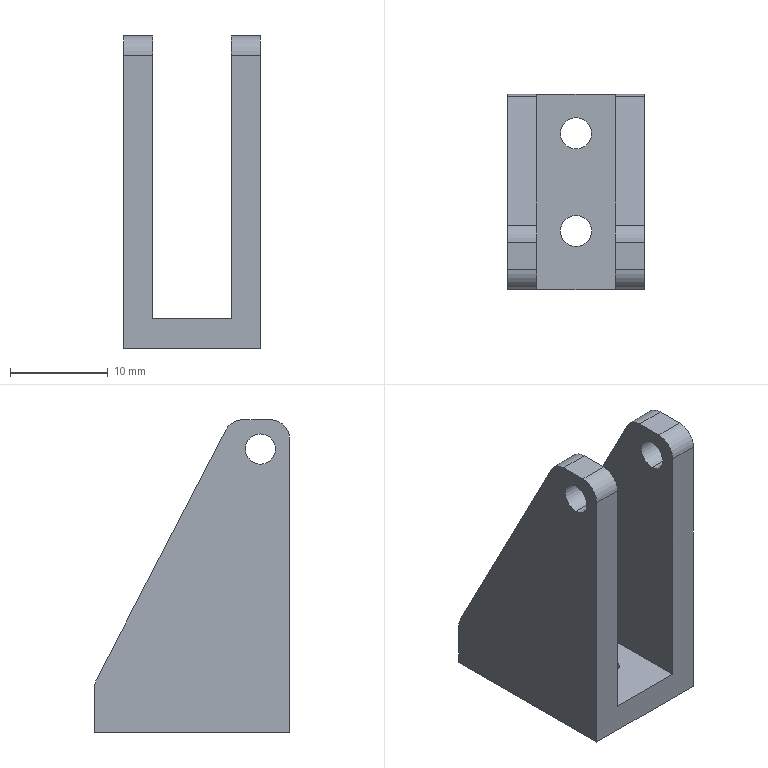Part | SolidWorks | features ICE 4, Extrusion 1, Fillet 1 | 1 solid | 26 faces | box 14 x 20 x 32 mm | volume 3086 mm3 | cylinder 14 | plane 12 | commonest cylinder face diameters 4 x6 3.1 x4 3.2 x4
STEP:
#1=CARTESIAN_POINT('',(-1.6,16.,-16.));
#2=VERTEX_POINT('',#1);
#3=CARTESIAN_POINT('',(1.6,16.,-16.));
#4=VERTEX_POINT('',#3);
#5=CARTESIAN_POINT('',(0.,16.,-16.));
#6=DIRECTION('',(0.,0.,1.));
#7=DIRECTION('',(1.,0.,0.));
#8=AXIS2_PLACEMENT_3D('',#5,#6,#7);
#9=CIRCLE('',#8,1.6);
#10=EDGE_CURVE('',#2,#4,#9,.T.);
#11=ORIENTED_EDGE('',*,*,#10,.F.);
#12=CARTESIAN_POINT('',(-1.6,16.,-13.));
#13=VERTEX_POINT('',#12);
#14=CARTESIAN_POINT('',(-1.6,16.,-33.));
#15=DIRECTION('',(0.,0.,1.));
#16=VECTOR('',#15,1000.);
#17=LINE('',#14,#16);
#18=EDGE_CURVE('',#2,#13,#17,.T.);
#19=ORIENTED_EDGE('',*,*,#18,.T.);
#20=CARTESIAN_POINT('',(1.6,16.,-13.));
#21=VERTEX_POINT('',#20);
#22=CARTESIAN_POINT('',(0.,16.,-13.));
#23=DIRECTION('',(0.,0.,1.));
#24=DIRECTION('',(1.,0.,0.));
#25=AXIS2_PLACEMENT_3D('',#22,#23,#24);
#26=CIRCLE('',#25,1.6);
#27=EDGE_CURVE('',#13,#21,#26,.T.);
#28=ORIENTED_EDGE('',*,*,#27,.T.);
#29=CARTESIAN_POINT('',(1.6,16.,-33.));
#30=DIRECTION('',(0.,0.,1.));
#31=VECTOR('',#30,1000.);
#32=LINE('',#29,#31);
#33=EDGE_CURVE('',#4,#21,#32,.T.);
#34=ORIENTED_EDGE('',*,*,#33,.F.);
#35=EDGE_LOOP('',(#11,#19,#28,#34));
#36=FACE_OUTER_BOUND('',#35,.T.);
#37=CARTESIAN_POINT('',(0.,16.,-33.));
#38=DIRECTION('',(0.,0.,1.));
#39=DIRECTION('',(1.,0.,0.));
#40=AXIS2_PLACEMENT_3D('',#37,#38,#39);
#41=CYLINDRICAL_SURFACE('',#40,1.6);
#42=ADVANCED_FACE('',(#36),#41,.F.);
#43=CARTESIAN_POINT('',(-1.6,6.,-16.));
#44=VERTEX_POINT('',#43);
#45=CARTESIAN_POINT('',(1.6,6.,-16.));
#46=VERTEX_POINT('',#45);
#47=CARTESIAN_POINT('',(0.,6.,-16.));
#48=DIRECTION('',(0.,0.,1.));
#49=DIRECTION('',(1.,0.,0.));
#50=AXIS2_PLACEMENT_3D('',#47,#48,#49);
#51=CIRCLE('',#50,1.6);
#52=EDGE_CURVE('',#44,#46,#51,.T.);
#53=ORIENTED_EDGE('',*,*,#52,.F.);
#54=CARTESIAN_POINT('',(-1.6,6.,-13.));
#55=VERTEX_POINT('',#54);
#56=CARTESIAN_POINT('',(-1.6,6.,-33.));
#57=DIRECTION('',(0.,0.,1.));
#58=VECTOR('',#57,1000.);
#59=LINE('',#56,#58);
#60=EDGE_CURVE('',#44,#55,#59,.T.);
#61=ORIENTED_EDGE('',*,*,#60,.T.);
#62=CARTESIAN_POINT('',(1.6,6.,-13.));
#63=VERTEX_POINT('',#62);
#64=CARTESIAN_POINT('',(0.,6.,-13.));
#65=DIRECTION('',(0.,0.,1.));
#66=DIRECTION('',(1.,0.,0.));
#67=AXIS2_PLACEMENT_3D('',#64,#65,#66);
#68=CIRCLE('',#67,1.6);
#69=EDGE_CURVE('',#55,#63,#68,.T.);
#70=ORIENTED_EDGE('',*,*,#69,.T.);
#71=CARTESIAN_POINT('',(1.6,6.,-33.));
#72=DIRECTION('',(0.,0.,1.));
#73=VECTOR('',#72,1000.);
#74=LINE('',#71,#73);
#75=EDGE_CURVE('',#46,#63,#74,.T.);
#76=ORIENTED_EDGE('',*,*,#75,.F.);
#77=EDGE_LOOP('',(#53,#61,#70,#76));
#78=FACE_OUTER_BOUND('',#77,.T.);
#79=CARTESIAN_POINT('',(0.,6.,-33.));
#80=DIRECTION('',(0.,0.,1.));
#81=DIRECTION('',(1.,0.,0.));
#82=AXIS2_PLACEMENT_3D('',#79,#80,#81);
#83=CYLINDRICAL_SURFACE('',#82,1.6);
#84=ADVANCED_FACE('',(#78),#83,.F.);
#85=CARTESIAN_POINT('',(7.,3.,11.45));
#86=VERTEX_POINT('',#85);
#87=CARTESIAN_POINT('',(7.,3.,14.55));
#88=VERTEX_POINT('',#87);
#89=CARTESIAN_POINT('',(7.,3.,13.));
#90=DIRECTION('',(-1.,0.,0.));
#91=DIRECTION('',(0.,0.,1.));
#92=AXIS2_PLACEMENT_3D('',#89,#90,#91);
#93=CIRCLE('',#92,1.55);
#94=EDGE_CURVE('',#86,#88,#93,.T.);
#95=ORIENTED_EDGE('',*,*,#94,.F.);
#96=CARTESIAN_POINT('',(4.,3.,11.45));
#97=VERTEX_POINT('',#96);
#98=CARTESIAN_POINT('',(13.,3.,11.45));
#99=DIRECTION('',(-1.,0.,0.));
#100=VECTOR('',#99,1000.);
#101=LINE('',#98,#100);
#102=EDGE_CURVE('',#86,#97,#101,.T.);
#103=ORIENTED_EDGE('',*,*,#102,.T.);
#104=CARTESIAN_POINT('',(4.,3.,14.55));
#105=VERTEX_POINT('',#104);
#106=CARTESIAN_POINT('',(4.,3.,13.));
#107=DIRECTION('',(1.,0.,0.));
#108=DIRECTION('',(0.,0.,-1.));
#109=AXIS2_PLACEMENT_3D('',#106,#107,#108);
#110=CIRCLE('',#109,1.55);
#111=EDGE_CURVE('',#105,#97,#110,.T.);
#112=ORIENTED_EDGE('',*,*,#111,.F.);
#113=CARTESIAN_POINT('',(13.,3.,14.55));
#114=DIRECTION('',(-1.,0.,0.));
#115=VECTOR('',#114,1000.);
#116=LINE('',#113,#115);
#117=EDGE_CURVE('',#88,#105,#116,.T.);
#118=ORIENTED_EDGE('',*,*,#117,.F.);
#119=EDGE_LOOP('',(#95,#103,#112,#118));
#120=FACE_OUTER_BOUND('',#119,.T.);
#121=CARTESIAN_POINT('',(13.,3.,13.));
#122=DIRECTION('',(-1.,0.,0.));
#123=DIRECTION('',(0.,0.,1.));
#124=AXIS2_PLACEMENT_3D('',#121,#122,#123);
#125=CYLINDRICAL_SURFACE('',#124,1.55);
#126=ADVANCED_FACE('',(#120),#125,.F.);
#127=CARTESIAN_POINT('',(-4.,3.,11.45));
#128=VERTEX_POINT('',#127);
#129=CARTESIAN_POINT('',(-4.,3.,14.55));
#130=VERTEX_POINT('',#129);
#131=CARTESIAN_POINT('',(-4.,3.,13.));
#132=DIRECTION('',(-1.,0.,0.));
#133=DIRECTION('',(0.,0.,1.));
#134=AXIS2_PLACEMENT_3D('',#131,#132,#133);
#135=CIRCLE('',#134,1.55);
#136=EDGE_CURVE('',#128,#130,#135,.T.);
#137=ORIENTED_EDGE('',*,*,#136,.F.);
#138=CARTESIAN_POINT('',(-7.,3.,11.45));
#139=VERTEX_POINT('',#138);
#140=CARTESIAN_POINT('',(13.,3.,11.45));
#141=DIRECTION('',(-1.,0.,0.));
#142=VECTOR('',#141,1000.);
#143=LINE('',#140,#142);
#144=EDGE_CURVE('',#128,#139,#143,.T.);
#145=ORIENTED_EDGE('',*,*,#144,.T.);
#146=CARTESIAN_POINT('',(-7.,3.,14.55));
#147=VERTEX_POINT('',#146);
#148=CARTESIAN_POINT('',(-7.,3.,13.));
#149=DIRECTION('',(-1.,0.,0.));
#150=DIRECTION('',(0.,0.,1.));
#151=AXIS2_PLACEMENT_3D('',#148,#149,#150);
#152=CIRCLE('',#151,1.55);
#153=EDGE_CURVE('',#139,#147,#152,.T.);
#154=ORIENTED_EDGE('',*,*,#153,.T.);
#155=CARTESIAN_POINT('',(13.,3.,14.55));
#156=DIRECTION('',(-1.,0.,0.));
#157=VECTOR('',#156,1000.);
#158=LINE('',#155,#157);
#159=EDGE_CURVE('',#130,#147,#158,.T.);
#160=ORIENTED_EDGE('',*,*,#159,.F.);
#161=EDGE_LOOP('',(#137,#145,#154,#160));
#162=FACE_OUTER_BOUND('',#161,.T.);
#163=CARTESIAN_POINT('',(13.,3.,13.));
#164=DIRECTION('',(-1.,0.,0.));
#165=DIRECTION('',(0.,0.,1.));
#166=AXIS2_PLACEMENT_3D('',#163,#164,#165);
#167=CYLINDRICAL_SURFACE('',#166,1.55);
#168=ADVANCED_FACE('',(#162),#167,.F.);
#169=CARTESIAN_POINT('',(7.,4.784,16.));
#170=VERTEX_POINT('',#169);
#171=CARTESIAN_POINT('',(7.,2.,16.));
#172=VERTEX_POINT('',#171);
#173=CARTESIAN_POINT('',(7.,20.,16.));
#174=DIRECTION('',(0.,-1.,0.));
#175=VECTOR('',#174,1000.);
#176=LINE('',#173,#175);
#177=EDGE_CURVE('',#170,#172,#176,.T.);
#178=ORIENTED_EDGE('',*,*,#177,.F.);
#179=CARTESIAN_POINT('',(4.,4.784,16.));
#180=VERTEX_POINT('',#179);
#181=CARTESIAN_POINT('',(-7.,4.784,16.));
#182=DIRECTION('',(-1.,0.,0.));
#183=VECTOR('',#182,1000.);
#184=LINE('',#181,#183);
#185=EDGE_CURVE('',#170,#180,#184,.T.);
#186=ORIENTED_EDGE('',*,*,#185,.T.);
#187=CARTESIAN_POINT('',(4.,2.,16.));
#188=VERTEX_POINT('',#187);
#189=CARTESIAN_POINT('',(4.,20.,16.));
#190=DIRECTION('',(0.,-1.,0.));
#191=VECTOR('',#190,1000.);
#192=LINE('',#189,#191);
#193=EDGE_CURVE('',#180,#188,#192,.T.);
#194=ORIENTED_EDGE('',*,*,#193,.T.);
#195=CARTESIAN_POINT('',(7.,2.,16.));
#196=DIRECTION('',(1.,0.,0.));
#197=VECTOR('',#196,1000.);
#198=LINE('',#195,#197);
#199=EDGE_CURVE('',#188,#172,#198,.T.);
#200=ORIENTED_EDGE('',*,*,#199,.T.);
#201=EDGE_LOOP('',(#178,#186,#194,#200));
#202=FACE_OUTER_BOUND('',#201,.T.);
#203=CARTESIAN_POINT('',(-7.,20.,16.));
#204=DIRECTION('',(0.,0.,-1.));
#205=DIRECTION('',(-1.,0.,0.));
#206=AXIS2_PLACEMENT_3D('',#203,#204,#205);
#207=PLANE('',#206);
#208=ADVANCED_FACE('',(#202),#207,.F.);
#209=CARTESIAN_POINT('',(7.,6.56,14.921));
#210=VERTEX_POINT('',#209);
#211=CARTESIAN_POINT('',(7.,19.776,-10.567));
#212=VERTEX_POINT('',#211);
#213=CARTESIAN_POINT('',(7.,6.,16.));
#214=DIRECTION('',(0.,0.4603,-0.8878));
#215=VECTOR('',#214,1000.);
#216=LINE('',#213,#215);
#217=EDGE_CURVE('',#210,#212,#216,.T.);
#218=ORIENTED_EDGE('',*,*,#217,.T.);
#219=CARTESIAN_POINT('',(4.,19.776,-10.567));
#220=VERTEX_POINT('',#219);
#221=CARTESIAN_POINT('',(-13.,19.776,-10.567));
#222=DIRECTION('',(-1.,0.,0.));
#223=VECTOR('',#222,1000.);
#224=LINE('',#221,#223);
#225=EDGE_CURVE('',#212,#220,#224,.T.);
#226=ORIENTED_EDGE('',*,*,#225,.T.);
#227=CARTESIAN_POINT('',(4.,6.56,14.921));
#228=VERTEX_POINT('',#227);
#229=CARTESIAN_POINT('',(4.,6.,16.));
#230=DIRECTION('',(0.,-0.4603,0.8878));
#231=VECTOR('',#230,1000.);
#232=LINE('',#229,#231);
#233=EDGE_CURVE('',#220,#228,#232,.T.);
#234=ORIENTED_EDGE('',*,*,#233,.T.);
#235=CARTESIAN_POINT('',(-13.,6.56,14.921));
#236=DIRECTION('',(1.,0.,0.));
#237=VECTOR('',#236,1000.);
#238=LINE('',#235,#237);
#239=EDGE_CURVE('',#228,#210,#238,.T.);
#240=ORIENTED_EDGE('',*,*,#239,.T.);
#241=EDGE_LOOP('',(#218,#226,#234,#240));
#242=FACE_OUTER_BOUND('',#241,.T.);
#243=CARTESIAN_POINT('',(-13.,6.,16.));
#244=DIRECTION('',(0.,-0.8878,-0.4603));
#245=DIRECTION('',(0.,0.4603,-0.8878));
#246=AXIS2_PLACEMENT_3D('',#243,#244,#245);
#247=PLANE('',#246);
#248=ADVANCED_FACE('',(#242),#247,.F.);
#249=CARTESIAN_POINT('',(7.,3.,13.));
#250=DIRECTION('',(-1.,0.,0.));
#251=DIRECTION('',(0.,0.,1.));
#252=AXIS2_PLACEMENT_3D('',#249,#250,#251);
#253=CIRCLE('',#252,1.55);
#254=EDGE_CURVE('',#88,#86,#253,.T.);
#255=ORIENTED_EDGE('',*,*,#254,.T.);
#256=ORIENTED_EDGE('',*,*,#94,.T.);
#257=EDGE_LOOP('',(#255,#256));
#258=FACE_BOUND('',#257,.T.);
#259=CARTESIAN_POINT('',(7.,20.,-11.488));
#260=VERTEX_POINT('',#259);
#261=CARTESIAN_POINT('',(7.,20.,-16.));
#262=VERTEX_POINT('',#261);
#263=CARTESIAN_POINT('',(7.,20.,16.));
#264=DIRECTION('',(0.,0.,-1.));
#265=VECTOR('',#264,1000.);
#266=LINE('',#263,#265);
#267=EDGE_CURVE('',#260,#262,#266,.T.);
#268=ORIENTED_EDGE('',*,*,#267,.F.);
#269=CARTESIAN_POINT('',(7.,18.,-11.488));
#270=DIRECTION('',(1.,0.,0.));
#271=DIRECTION('',(0.,0.,1.));
#272=AXIS2_PLACEMENT_3D('',#269,#270,#271);
#273=CIRCLE('',#272,2.);
#274=EDGE_CURVE('',#260,#212,#273,.T.);
#275=ORIENTED_EDGE('',*,*,#274,.T.);
#276=ORIENTED_EDGE('',*,*,#217,.F.);
#277=CARTESIAN_POINT('',(7.,4.784,14.));
#278=DIRECTION('',(1.,0.,0.));
#279=DIRECTION('',(0.,0.,1.));
#280=AXIS2_PLACEMENT_3D('',#277,#278,#279);
#281=CIRCLE('',#280,2.);
#282=EDGE_CURVE('',#210,#170,#281,.T.);
#283=ORIENTED_EDGE('',*,*,#282,.T.);
#284=ORIENTED_EDGE('',*,*,#177,.T.);
#285=CARTESIAN_POINT('',(7.,0.,14.));
#286=VERTEX_POINT('',#285);
#287=CARTESIAN_POINT('',(7.,2.,14.));
#288=DIRECTION('',(1.,0.,0.));
#289=DIRECTION('',(0.,0.,1.));
#290=AXIS2_PLACEMENT_3D('',#287,#288,#289);
#291=CIRCLE('',#290,2.);
#292=EDGE_CURVE('',#172,#286,#291,.T.);
#293=ORIENTED_EDGE('',*,*,#292,.T.);
#294=CARTESIAN_POINT('',(7.,0.,-16.));
#295=VERTEX_POINT('',#294);
#296=CARTESIAN_POINT('',(7.,0.,16.));
#297=DIRECTION('',(0.,0.,-1.));
#298=VECTOR('',#297,1000.);
#299=LINE('',#296,#298);
#300=EDGE_CURVE('',#286,#295,#299,.T.);
#301=ORIENTED_EDGE('',*,*,#300,.T.);
#302=CARTESIAN_POINT('',(7.,20.,-16.));
#303=DIRECTION('',(0.,-1.,0.));
#304=VECTOR('',#303,1000.);
#305=LINE('',#302,#304);
#306=EDGE_CURVE('',#262,#295,#305,.T.);
#307=ORIENTED_EDGE('',*,*,#306,.F.);
#308=EDGE_LOOP('',(#268,#275,#276,#283,#284,#293,#301,#307));
#309=FACE_OUTER_BOUND('',#308,.T.);
#310=CARTESIAN_POINT('',(7.,20.,16.));
#311=DIRECTION('',(-1.,0.,0.));
#312=DIRECTION('',(0.,0.,1.));
#313=AXIS2_PLACEMENT_3D('',#310,#311,#312);
#314=PLANE('',#313);
#315=ADVANCED_FACE('',(#258,#309),#314,.F.);
#316=CARTESIAN_POINT('',(0.,16.,-16.));
#317=DIRECTION('',(0.,0.,1.));
#318=DIRECTION('',(1.,0.,0.));
#319=AXIS2_PLACEMENT_3D('',#316,#317,#318);
#320=CIRCLE('',#319,1.6);
#321=EDGE_CURVE('',#4,#2,#320,.T.);
#322=ORIENTED_EDGE('',*,*,#321,.T.);
#323=ORIENTED_EDGE('',*,*,#10,.T.);
#324=EDGE_LOOP('',(#322,#323));
#325=FACE_BOUND('',#324,.T.);
#326=CARTESIAN_POINT('',(0.,6.,-16.));
#327=DIRECTION('',(0.,0.,1.));
#328=DIRECTION('',(1.,0.,0.));
#329=AXIS2_PLACEMENT_3D('',#326,#327,#328);
#330=CIRCLE('',#329,1.6);
#331=EDGE_CURVE('',#46,#44,#330,.T.);
#332=ORIENTED_EDGE('',*,*,#331,.T.);
#333=ORIENTED_EDGE('',*,*,#52,.T.);
#334=EDGE_LOOP('',(#332,#333));
#335=FACE_BOUND('',#334,.T.);
#336=CARTESIAN_POINT('',(-7.,0.,-16.));
#337=VERTEX_POINT('',#336);
#338=CARTESIAN_POINT('',(-7.,0.,-16.));
#339=DIRECTION('',(-1.,0.,0.));
#340=VECTOR('',#339,1000.);
#341=LINE('',#338,#340);
#342=EDGE_CURVE('',#295,#337,#341,.T.);
#343=ORIENTED_EDGE('',*,*,#342,.T.);
#344=CARTESIAN_POINT('',(-7.,20.,-16.));
#345=VERTEX_POINT('',#344);
#346=CARTESIAN_POINT('',(-7.,20.,-16.));
#347=DIRECTION('',(0.,-1.,0.));
#348=VECTOR('',#347,1000.);
#349=LINE('',#346,#348);
#350=EDGE_CURVE('',#345,#337,#349,.T.);
#351=ORIENTED_EDGE('',*,*,#350,.F.);
#352=CARTESIAN_POINT('',(-7.,20.,-16.));
#353=DIRECTION('',(-1.,0.,0.));
#354=VECTOR('',#353,1000.);
#355=LINE('',#352,#354);
#356=EDGE_CURVE('',#262,#345,#355,.T.);
#357=ORIENTED_EDGE('',*,*,#356,.F.);
#358=ORIENTED_EDGE('',*,*,#306,.T.);
#359=EDGE_LOOP('',(#343,#351,#357,#358));
#360=FACE_OUTER_BOUND('',#359,.T.);
#361=CARTESIAN_POINT('',(-7.,20.,-16.));
#362=DIRECTION('',(0.,0.,1.));
#363=DIRECTION('',(1.,0.,0.));
#364=AXIS2_PLACEMENT_3D('',#361,#362,#363);
#365=PLANE('',#364);
#366=ADVANCED_FACE('',(#325,#335,#360),#365,.F.);
#367=CARTESIAN_POINT('',(-7.,3.,13.));
#368=DIRECTION('',(-1.,0.,0.));
#369=DIRECTION('',(0.,0.,1.));
#370=AXIS2_PLACEMENT_3D('',#367,#368,#369);
#371=CIRCLE('',#370,1.55);
#372=EDGE_CURVE('',#147,#139,#371,.T.);
#373=ORIENTED_EDGE('',*,*,#372,.F.);
#374=ORIENTED_EDGE('',*,*,#153,.F.);
#375=EDGE_LOOP('',(#373,#374));
#376=FACE_BOUND('',#375,.T.);
#377=CARTESIAN_POINT('',(-7.,0.,14.));
#378=VERTEX_POINT('',#377);
#379=CARTESIAN_POINT('',(-7.,0.,16.));
#380=DIRECTION('',(0.,0.,1.));
#381=VECTOR('',#380,1000.);
#382=LINE('',#379,#381);
#383=EDGE_CURVE('',#337,#378,#382,.T.);
#384=ORIENTED_EDGE('',*,*,#383,.T.);
#385=CARTESIAN_POINT('',(-7.,2.,16.));
#386=VERTEX_POINT('',#385);
#387=CARTESIAN_POINT('',(-7.,2.,14.));
#388=DIRECTION('',(-1.,0.,0.));
#389=DIRECTION('',(0.,0.,-1.));
#390=AXIS2_PLACEMENT_3D('',#387,#388,#389);
#391=CIRCLE('',#390,2.);
#392=EDGE_CURVE('',#378,#386,#391,.T.);
#393=ORIENTED_EDGE('',*,*,#392,.T.);
#394=CARTESIAN_POINT('',(-7.,4.784,16.));
#395=VERTEX_POINT('',#394);
#396=CARTESIAN_POINT('',(-7.,20.,16.));
#397=DIRECTION('',(0.,-1.,0.));
#398=VECTOR('',#397,1000.);
#399=LINE('',#396,#398);
#400=EDGE_CURVE('',#395,#386,#399,.T.);
#401=ORIENTED_EDGE('',*,*,#400,.F.);
#402=CARTESIAN_POINT('',(-7.,6.56,14.921));
#403=VERTEX_POINT('',#402);
#404=CARTESIAN_POINT('',(-7.,4.784,14.));
#405=DIRECTION('',(-1.,0.,0.));
#406=DIRECTION('',(0.,0.,-1.));
#407=AXIS2_PLACEMENT_3D('',#404,#405,#406);
#408=CIRCLE('',#407,2.);
#409=EDGE_CURVE('',#395,#403,#408,.T.);
#410=ORIENTED_EDGE('',*,*,#409,.T.);
#411=CARTESIAN_POINT('',(-7.,19.776,-10.567));
#412=VERTEX_POINT('',#411);
#413=CARTESIAN_POINT('',(-7.,8.966,10.279));
#414=DIRECTION('',(0.,0.4603,-0.8878));
#415=VECTOR('',#414,1000.);
#416=LINE('',#413,#415);
#417=EDGE_CURVE('',#403,#412,#416,.T.);
#418=ORIENTED_EDGE('',*,*,#417,.T.);
#419=CARTESIAN_POINT('',(-7.,20.,-11.488));
#420=VERTEX_POINT('',#419);
#421=CARTESIAN_POINT('',(-7.,18.,-11.488));
#422=DIRECTION('',(-1.,0.,0.));
#423=DIRECTION('',(0.,0.,-1.));
#424=AXIS2_PLACEMENT_3D('',#421,#422,#423);
#425=CIRCLE('',#424,2.);
#426=EDGE_CURVE('',#412,#420,#425,.T.);
#427=ORIENTED_EDGE('',*,*,#426,.T.);
#428=CARTESIAN_POINT('',(-7.,20.,16.));
#429=DIRECTION('',(0.,0.,1.));
#430=VECTOR('',#429,1000.);
#431=LINE('',#428,#430);
#432=EDGE_CURVE('',#345,#420,#431,.T.);
#433=ORIENTED_EDGE('',*,*,#432,.F.);
#434=ORIENTED_EDGE('',*,*,#350,.T.);
#435=EDGE_LOOP('',(#384,#393,#401,#410,#418,#427,#433,#434));
#436=FACE_OUTER_BOUND('',#435,.T.);
#437=CARTESIAN_POINT('',(-7.,20.,16.));
#438=DIRECTION('',(1.,0.,0.));
#439=DIRECTION('',(0.,0.,-1.));
#440=AXIS2_PLACEMENT_3D('',#437,#438,#439);
#441=PLANE('',#440);
#442=ADVANCED_FACE('',(#376,#436),#441,.F.);
#443=ORIENTED_EDGE('',*,*,#400,.T.);
#444=CARTESIAN_POINT('',(-4.,2.,16.));
#445=VERTEX_POINT('',#444);
#446=CARTESIAN_POINT('',(-4.,2.,16.));
#447=DIRECTION('',(1.,0.,0.));
#448=VECTOR('',#447,1000.);
#449=LINE('',#446,#448);
#450=EDGE_CURVE('',#386,#445,#449,.T.);
#451=ORIENTED_EDGE('',*,*,#450,.T.);
#452=CARTESIAN_POINT('',(-4.,4.784,16.));
#453=VERTEX_POINT('',#452);
#454=CARTESIAN_POINT('',(-4.,20.,16.));
#455=DIRECTION('',(0.,-1.,0.));
#456=VECTOR('',#455,1000.);
#457=LINE('',#454,#456);
#458=EDGE_CURVE('',#453,#445,#457,.T.);
#459=ORIENTED_EDGE('',*,*,#458,.F.);
#460=CARTESIAN_POINT('',(-7.,4.784,16.));
#461=DIRECTION('',(-1.,0.,0.));
#462=VECTOR('',#461,1000.);
#463=LINE('',#460,#462);
#464=EDGE_CURVE('',#453,#395,#463,.T.);
#465=ORIENTED_EDGE('',*,*,#464,.T.);
#466=EDGE_LOOP('',(#443,#451,#459,#465));
#467=FACE_OUTER_BOUND('',#466,.T.);
#468=CARTESIAN_POINT('',(-7.,20.,16.));
#469=DIRECTION('',(0.,0.,-1.));
#470=DIRECTION('',(-1.,0.,0.));
#471=AXIS2_PLACEMENT_3D('',#468,#469,#470);
#472=PLANE('',#471);
#473=ADVANCED_FACE('',(#467),#472,.F.);
#474=CARTESIAN_POINT('',(4.,20.,-13.));
#475=VERTEX_POINT('',#474);
#476=CARTESIAN_POINT('',(4.,20.,-11.488));
#477=VERTEX_POINT('',#476);
#478=CARTESIAN_POINT('',(4.,20.,16.));
#479=DIRECTION('',(0.,0.,1.));
#480=VECTOR('',#479,1000.);
#481=LINE('',#478,#480);
#482=EDGE_CURVE('',#475,#477,#481,.T.);
#483=ORIENTED_EDGE('',*,*,#482,.T.);
#484=CARTESIAN_POINT('',(0.,20.,-11.488));
#485=DIRECTION('',(1.,0.,0.));
#486=VECTOR('',#485,1000.);
#487=LINE('',#484,#486);
#488=EDGE_CURVE('',#477,#260,#487,.T.);
#489=ORIENTED_EDGE('',*,*,#488,.T.);
#490=ORIENTED_EDGE('',*,*,#267,.T.);
#491=ORIENTED_EDGE('',*,*,#356,.T.);
#492=ORIENTED_EDGE('',*,*,#432,.T.);
#493=CARTESIAN_POINT('',(-4.,20.,-11.488));
#494=VERTEX_POINT('',#493);
#495=CARTESIAN_POINT('',(0.,20.,-11.488));
#496=DIRECTION('',(1.,0.,0.));
#497=VECTOR('',#496,1000.);
#498=LINE('',#495,#497);
#499=EDGE_CURVE('',#420,#494,#498,.T.);
#500=ORIENTED_EDGE('',*,*,#499,.T.);
#501=CARTESIAN_POINT('',(-4.,20.,-13.));
#502=VERTEX_POINT('',#501);
#503=CARTESIAN_POINT('',(-4.,20.,16.));
#504=DIRECTION('',(0.,0.,-1.));
#505=VECTOR('',#504,1000.);
#506=LINE('',#503,#505);
#507=EDGE_CURVE('',#494,#502,#506,.T.);
#508=ORIENTED_EDGE('',*,*,#507,.T.);
#509=CARTESIAN_POINT('',(4.,20.,-13.));
#510=DIRECTION('',(1.,0.,0.));
#511=VECTOR('',#510,1000.);
#512=LINE('',#509,#511);
#513=EDGE_CURVE('',#502,#475,#512,.T.);
#514=ORIENTED_EDGE('',*,*,#513,.T.);
#515=EDGE_LOOP('',(#483,#489,#490,#491,#492,#500,#508,#514));
#516=FACE_OUTER_BOUND('',#515,.T.);
#517=CARTESIAN_POINT('',(0.,20.,0.));
#518=DIRECTION('',(0.,-1.,0.));
#519=DIRECTION('',(0.,0.,-1.));
#520=AXIS2_PLACEMENT_3D('',#517,#518,#519);
#521=PLANE('',#520);
#522=ADVANCED_FACE('',(#516),#521,.F.);
#523=ORIENTED_EDGE('',*,*,#300,.F.);
#524=CARTESIAN_POINT('',(4.,0.,14.));
#525=VERTEX_POINT('',#524);
#526=CARTESIAN_POINT('',(4.,0.,14.));
#527=DIRECTION('',(-1.,0.,0.));
#528=VECTOR('',#527,1000.);
#529=LINE('',#526,#528);
#530=EDGE_CURVE('',#286,#525,#529,.T.);
#531=ORIENTED_EDGE('',*,*,#530,.T.);
#532=CARTESIAN_POINT('',(4.,0.,-13.));
#533=VERTEX_POINT('',#532);
#534=CARTESIAN_POINT('',(4.,0.,16.));
#535=DIRECTION('',(0.,0.,1.));
#536=VECTOR('',#535,1000.);
#537=LINE('',#534,#536);
#538=EDGE_CURVE('',#533,#525,#537,.T.);
#539=ORIENTED_EDGE('',*,*,#538,.F.);
#540=CARTESIAN_POINT('',(-4.,0.,-13.));
#541=VERTEX_POINT('',#540);
#542=CARTESIAN_POINT('',(4.,0.,-13.));
#543=DIRECTION('',(1.,0.,0.));
#544=VECTOR('',#543,1000.);
#545=LINE('',#542,#544);
#546=EDGE_CURVE('',#541,#533,#545,.T.);
#547=ORIENTED_EDGE('',*,*,#546,.F.);
#548=CARTESIAN_POINT('',(-4.,0.,14.));
#549=VERTEX_POINT('',#548);
#550=CARTESIAN_POINT('',(-4.,0.,16.));
#551=DIRECTION('',(0.,0.,-1.));
#552=VECTOR('',#551,1000.);
#553=LINE('',#550,#552);
#554=EDGE_CURVE('',#549,#541,#553,.T.);
#555=ORIENTED_EDGE('',*,*,#554,.F.);
#556=CARTESIAN_POINT('',(-7.,0.,14.));
#557=DIRECTION('',(-1.,0.,0.));
#558=VECTOR('',#557,1000.);
#559=LINE('',#556,#558);
#560=EDGE_CURVE('',#549,#378,#559,.T.);
#561=ORIENTED_EDGE('',*,*,#560,.T.);
#562=ORIENTED_EDGE('',*,*,#383,.F.);
#563=ORIENTED_EDGE('',*,*,#342,.F.);
#564=EDGE_LOOP('',(#523,#531,#539,#547,#555,#561,#562,#563));
#565=FACE_OUTER_BOUND('',#564,.T.);
#566=CARTESIAN_POINT('',(0.,0.,0.));
#567=DIRECTION('',(0.,-1.,0.));
#568=DIRECTION('',(0.,0.,-1.));
#569=AXIS2_PLACEMENT_3D('',#566,#567,#568);
#570=PLANE('',#569);
#571=ADVANCED_FACE('',(#565),#570,.T.);
#572=CARTESIAN_POINT('',(-4.,6.56,14.921));
#573=VERTEX_POINT('',#572);
#574=CARTESIAN_POINT('',(-4.,19.776,-10.567));
#575=VERTEX_POINT('',#574);
#576=CARTESIAN_POINT('',(-4.,6.,16.));
#577=DIRECTION('',(0.,0.4603,-0.8878));
#578=VECTOR('',#577,1000.);
#579=LINE('',#576,#578);
#580=EDGE_CURVE('',#573,#575,#579,.T.);
#581=ORIENTED_EDGE('',*,*,#580,.T.);
#582=CARTESIAN_POINT('',(-13.,19.776,-10.567));
#583=DIRECTION('',(-1.,0.,0.));
#584=VECTOR('',#583,1000.);
#585=LINE('',#582,#584);
#586=EDGE_CURVE('',#575,#412,#585,.T.);
#587=ORIENTED_EDGE('',*,*,#586,.T.);
#588=ORIENTED_EDGE('',*,*,#417,.F.);
#589=CARTESIAN_POINT('',(-13.,6.56,14.921));
#590=DIRECTION('',(1.,0.,0.));
#591=VECTOR('',#590,1000.);
#592=LINE('',#589,#591);
#593=EDGE_CURVE('',#403,#573,#592,.T.);
#594=ORIENTED_EDGE('',*,*,#593,.T.);
#595=EDGE_LOOP('',(#581,#587,#588,#594));
#596=FACE_OUTER_BOUND('',#595,.T.);
#597=CARTESIAN_POINT('',(-13.,6.,16.));
#598=DIRECTION('',(0.,-0.8878,-0.4603));
#599=DIRECTION('',(0.,0.4603,-0.8878));
#600=AXIS2_PLACEMENT_3D('',#597,#598,#599);
#601=PLANE('',#600);
#602=ADVANCED_FACE('',(#596),#601,.F.);
#603=ORIENTED_EDGE('',*,*,#111,.T.);
#604=CARTESIAN_POINT('',(4.,3.,13.));
#605=DIRECTION('',(1.,0.,0.));
#606=DIRECTION('',(0.,0.,-1.));
#607=AXIS2_PLACEMENT_3D('',#604,#605,#606);
#608=CIRCLE('',#607,1.55);
#609=EDGE_CURVE('',#97,#105,#608,.T.);
#610=ORIENTED_EDGE('',*,*,#609,.T.);
#611=EDGE_LOOP('',(#603,#610));
#612=FACE_BOUND('',#611,.T.);
#613=ORIENTED_EDGE('',*,*,#233,.F.);
#614=CARTESIAN_POINT('',(4.,18.,-11.488));
#615=DIRECTION('',(-1.,0.,0.));
#616=DIRECTION('',(0.,0.,-1.));
#617=AXIS2_PLACEMENT_3D('',#614,#615,#616);
#618=CIRCLE('',#617,2.);
#619=EDGE_CURVE('',#220,#477,#618,.T.);
#620=ORIENTED_EDGE('',*,*,#619,.T.);
#621=ORIENTED_EDGE('',*,*,#482,.F.);
#622=CARTESIAN_POINT('',(4.,20.,-13.));
#623=DIRECTION('',(0.,-1.,0.));
#624=VECTOR('',#623,1000.);
#625=LINE('',#622,#624);
#626=EDGE_CURVE('',#475,#533,#625,.T.);
#627=ORIENTED_EDGE('',*,*,#626,.T.);
#628=ORIENTED_EDGE('',*,*,#538,.T.);
#629=CARTESIAN_POINT('',(4.,2.,14.));
#630=DIRECTION('',(-1.,0.,0.));
#631=DIRECTION('',(0.,0.,-1.));
#632=AXIS2_PLACEMENT_3D('',#629,#630,#631);
#633=CIRCLE('',#632,2.);
#634=EDGE_CURVE('',#525,#188,#633,.T.);
#635=ORIENTED_EDGE('',*,*,#634,.T.);
#636=ORIENTED_EDGE('',*,*,#193,.F.);
#637=CARTESIAN_POINT('',(4.,4.784,14.));
#638=DIRECTION('',(-1.,0.,0.));
#639=DIRECTION('',(0.,0.,-1.));
#640=AXIS2_PLACEMENT_3D('',#637,#638,#639);
#641=CIRCLE('',#640,2.);
#642=EDGE_CURVE('',#180,#228,#641,.T.);
#643=ORIENTED_EDGE('',*,*,#642,.T.);
#644=EDGE_LOOP('',(#613,#620,#621,#627,#628,#635,#636,#643));
#645=FACE_OUTER_BOUND('',#644,.T.);
#646=CARTESIAN_POINT('',(4.,20.,16.));
#647=DIRECTION('',(1.,0.,0.));
#648=DIRECTION('',(0.,0.,-1.));
#649=AXIS2_PLACEMENT_3D('',#646,#647,#648);
#650=PLANE('',#649);
#651=ADVANCED_FACE('',(#612,#645),#650,.F.);
#652=CARTESIAN_POINT('',(-4.,3.,13.));
#653=DIRECTION('',(-1.,0.,0.));
#654=DIRECTION('',(0.,0.,1.));
#655=AXIS2_PLACEMENT_3D('',#652,#653,#654);
#656=CIRCLE('',#655,1.55);
#657=EDGE_CURVE('',#130,#128,#656,.T.);
#658=ORIENTED_EDGE('',*,*,#657,.T.);
#659=ORIENTED_EDGE('',*,*,#136,.T.);
#660=EDGE_LOOP('',(#658,#659));
#661=FACE_BOUND('',#660,.T.);
#662=ORIENTED_EDGE('',*,*,#458,.T.);
#663=CARTESIAN_POINT('',(-4.,2.,14.));
#664=DIRECTION('',(1.,0.,0.));
#665=DIRECTION('',(0.,0.,1.));
#666=AXIS2_PLACEMENT_3D('',#663,#664,#665);
#667=CIRCLE('',#666,2.);
#668=EDGE_CURVE('',#445,#549,#667,.T.);
#669=ORIENTED_EDGE('',*,*,#668,.T.);
#670=ORIENTED_EDGE('',*,*,#554,.T.);
#671=CARTESIAN_POINT('',(-4.,20.,-13.));
#672=DIRECTION('',(0.,-1.,0.));
#673=VECTOR('',#672,1000.);
#674=LINE('',#671,#673);
#675=EDGE_CURVE('',#502,#541,#674,.T.);
#676=ORIENTED_EDGE('',*,*,#675,.F.);
#677=ORIENTED_EDGE('',*,*,#507,.F.);
#678=CARTESIAN_POINT('',(-4.,18.,-11.488));
#679=DIRECTION('',(1.,0.,0.));
#680=DIRECTION('',(0.,0.,1.));
#681=AXIS2_PLACEMENT_3D('',#678,#679,#680);
#682=CIRCLE('',#681,2.);
#683=EDGE_CURVE('',#494,#575,#682,.T.);
#684=ORIENTED_EDGE('',*,*,#683,.T.);
#685=ORIENTED_EDGE('',*,*,#580,.F.);
#686=CARTESIAN_POINT('',(-4.,4.784,14.));
#687=DIRECTION('',(1.,0.,0.));
#688=DIRECTION('',(0.,0.,1.));
#689=AXIS2_PLACEMENT_3D('',#686,#687,#688);
#690=CIRCLE('',#689,2.);
#691=EDGE_CURVE('',#573,#453,#690,.T.);
#692=ORIENTED_EDGE('',*,*,#691,.T.);
#693=EDGE_LOOP('',(#662,#669,#670,#676,#677,#684,#685,#692));
#694=FACE_OUTER_BOUND('',#693,.T.);
#695=CARTESIAN_POINT('',(-4.,20.,16.));
#696=DIRECTION('',(-1.,0.,0.));
#697=DIRECTION('',(0.,0.,1.));
#698=AXIS2_PLACEMENT_3D('',#695,#696,#697);
#699=PLANE('',#698);
#700=ADVANCED_FACE('',(#661,#694),#699,.F.);
#701=CARTESIAN_POINT('',(0.,16.,-13.));
#702=DIRECTION('',(0.,0.,1.));
#703=DIRECTION('',(1.,0.,0.));
#704=AXIS2_PLACEMENT_3D('',#701,#702,#703);
#705=CIRCLE('',#704,1.6);
#706=EDGE_CURVE('',#21,#13,#705,.T.);
#707=ORIENTED_EDGE('',*,*,#706,.F.);
#708=ORIENTED_EDGE('',*,*,#27,.F.);
#709=EDGE_LOOP('',(#707,#708));
#710=FACE_BOUND('',#709,.T.);
#711=CARTESIAN_POINT('',(0.,6.,-13.));
#712=DIRECTION('',(0.,0.,1.));
#713=DIRECTION('',(1.,0.,0.));
#714=AXIS2_PLACEMENT_3D('',#711,#712,#713);
#715=CIRCLE('',#714,1.6);
#716=EDGE_CURVE('',#63,#55,#715,.T.);
#717=ORIENTED_EDGE('',*,*,#716,.F.);
#718=ORIENTED_EDGE('',*,*,#69,.F.);
#719=EDGE_LOOP('',(#717,#718));
#720=FACE_BOUND('',#719,.T.);
#721=ORIENTED_EDGE('',*,*,#546,.T.);
#722=ORIENTED_EDGE('',*,*,#626,.F.);
#723=ORIENTED_EDGE('',*,*,#513,.F.);
#724=ORIENTED_EDGE('',*,*,#675,.T.);
#725=EDGE_LOOP('',(#721,#722,#723,#724));
#726=FACE_OUTER_BOUND('',#725,.T.);
#727=CARTESIAN_POINT('',(4.,20.,-13.));
#728=DIRECTION('',(0.,0.,-1.));
#729=DIRECTION('',(-1.,0.,0.));
#730=AXIS2_PLACEMENT_3D('',#727,#728,#729);
#731=PLANE('',#730);
#732=ADVANCED_FACE('',(#710,#720,#726),#731,.F.);
#733=ORIENTED_EDGE('',*,*,#619,.F.);
#734=ORIENTED_EDGE('',*,*,#225,.F.);
#735=ORIENTED_EDGE('',*,*,#274,.F.);
#736=ORIENTED_EDGE('',*,*,#488,.F.);
#737=EDGE_LOOP('',(#733,#734,#735,#736));
#738=FACE_OUTER_BOUND('',#737,.T.);
#739=CARTESIAN_POINT('',(0.,18.,-11.488));
#740=DIRECTION('',(1.,0.,0.));
#741=DIRECTION('',(0.,0.,-1.));
#742=AXIS2_PLACEMENT_3D('',#739,#740,#741);
#743=CYLINDRICAL_SURFACE('',#742,2.);
#744=ADVANCED_FACE('',(#738),#743,.T.);
#745=ORIENTED_EDGE('',*,*,#642,.F.);
#746=ORIENTED_EDGE('',*,*,#185,.F.);
#747=ORIENTED_EDGE('',*,*,#282,.F.);
#748=ORIENTED_EDGE('',*,*,#239,.F.);
#749=EDGE_LOOP('',(#745,#746,#747,#748));
#750=FACE_OUTER_BOUND('',#749,.T.);
#751=CARTESIAN_POINT('',(-13.,4.784,14.));
#752=DIRECTION('',(1.,0.,0.));
#753=DIRECTION('',(0.,0.,-1.));
#754=AXIS2_PLACEMENT_3D('',#751,#752,#753);
#755=CYLINDRICAL_SURFACE('',#754,2.);
#756=ADVANCED_FACE('',(#750),#755,.T.);
#757=ORIENTED_EDGE('',*,*,#634,.F.);
#758=ORIENTED_EDGE('',*,*,#530,.F.);
#759=ORIENTED_EDGE('',*,*,#292,.F.);
#760=ORIENTED_EDGE('',*,*,#199,.F.);
#761=EDGE_LOOP('',(#757,#758,#759,#760));
#762=FACE_OUTER_BOUND('',#761,.T.);
#763=CARTESIAN_POINT('',(-7.,2.,14.));
#764=DIRECTION('',(-1.,0.,0.));
#765=DIRECTION('',(0.,0.,1.));
#766=AXIS2_PLACEMENT_3D('',#763,#764,#765);
#767=CYLINDRICAL_SURFACE('',#766,2.);
#768=ADVANCED_FACE('',(#762),#767,.T.);
#769=ORIENTED_EDGE('',*,*,#392,.F.);
#770=ORIENTED_EDGE('',*,*,#560,.F.);
#771=ORIENTED_EDGE('',*,*,#668,.F.);
#772=ORIENTED_EDGE('',*,*,#450,.F.);
#773=EDGE_LOOP('',(#769,#770,#771,#772));
#774=FACE_OUTER_BOUND('',#773,.T.);
#775=CARTESIAN_POINT('',(-7.,2.,14.));
#776=DIRECTION('',(-1.,0.,0.));
#777=DIRECTION('',(0.,0.,1.));
#778=AXIS2_PLACEMENT_3D('',#775,#776,#777);
#779=CYLINDRICAL_SURFACE('',#778,2.);
#780=ADVANCED_FACE('',(#774),#779,.T.);
#781=ORIENTED_EDGE('',*,*,#426,.F.);
#782=ORIENTED_EDGE('',*,*,#586,.F.);
#783=ORIENTED_EDGE('',*,*,#683,.F.);
#784=ORIENTED_EDGE('',*,*,#499,.F.);
#785=EDGE_LOOP('',(#781,#782,#783,#784));
#786=FACE_OUTER_BOUND('',#785,.T.);
#787=CARTESIAN_POINT('',(0.,18.,-11.488));
#788=DIRECTION('',(1.,0.,0.));
#789=DIRECTION('',(0.,0.,-1.));
#790=AXIS2_PLACEMENT_3D('',#787,#788,#789);
#791=CYLINDRICAL_SURFACE('',#790,2.);
#792=ADVANCED_FACE('',(#786),#791,.T.);
#793=ORIENTED_EDGE('',*,*,#409,.F.);
#794=ORIENTED_EDGE('',*,*,#464,.F.);
#795=ORIENTED_EDGE('',*,*,#691,.F.);
#796=ORIENTED_EDGE('',*,*,#593,.F.);
#797=EDGE_LOOP('',(#793,#794,#795,#796));
#798=FACE_OUTER_BOUND('',#797,.T.);
#799=CARTESIAN_POINT('',(-13.,4.784,14.));
#800=DIRECTION('',(1.,0.,0.));
#801=DIRECTION('',(0.,0.,-1.));
#802=AXIS2_PLACEMENT_3D('',#799,#800,#801);
#803=CYLINDRICAL_SURFACE('',#802,2.);
#804=ADVANCED_FACE('',(#798),#803,.T.);
#805=ORIENTED_EDGE('',*,*,#144,.F.);
#806=ORIENTED_EDGE('',*,*,#657,.F.);
#807=ORIENTED_EDGE('',*,*,#159,.T.);
#808=ORIENTED_EDGE('',*,*,#372,.T.);
#809=EDGE_LOOP('',(#805,#806,#807,#808));
#810=FACE_OUTER_BOUND('',#809,.T.);
#811=CARTESIAN_POINT('',(13.,3.,13.));
#812=DIRECTION('',(-1.,0.,0.));
#813=DIRECTION('',(0.,0.,1.));
#814=AXIS2_PLACEMENT_3D('',#811,#812,#813);
#815=CYLINDRICAL_SURFACE('',#814,1.55);
#816=ADVANCED_FACE('',(#810),#815,.F.);
#817=ORIENTED_EDGE('',*,*,#102,.F.);
#818=ORIENTED_EDGE('',*,*,#254,.F.);
#819=ORIENTED_EDGE('',*,*,#117,.T.);
#820=ORIENTED_EDGE('',*,*,#609,.F.);
#821=EDGE_LOOP('',(#817,#818,#819,#820));
#822=FACE_OUTER_BOUND('',#821,.T.);
#823=CARTESIAN_POINT('',(13.,3.,13.));
#824=DIRECTION('',(-1.,0.,0.));
#825=DIRECTION('',(0.,0.,1.));
#826=AXIS2_PLACEMENT_3D('',#823,#824,#825);
#827=CYLINDRICAL_SURFACE('',#826,1.55);
#828=ADVANCED_FACE('',(#822),#827,.F.);
#829=ORIENTED_EDGE('',*,*,#60,.F.);
#830=ORIENTED_EDGE('',*,*,#331,.F.);
#831=ORIENTED_EDGE('',*,*,#75,.T.);
#832=ORIENTED_EDGE('',*,*,#716,.T.);
#833=EDGE_LOOP('',(#829,#830,#831,#832));
#834=FACE_OUTER_BOUND('',#833,.T.);
#835=CARTESIAN_POINT('',(0.,6.,-33.));
#836=DIRECTION('',(0.,0.,1.));
#837=DIRECTION('',(1.,0.,0.));
#838=AXIS2_PLACEMENT_3D('',#835,#836,#837);
#839=CYLINDRICAL_SURFACE('',#838,1.6);
#840=ADVANCED_FACE('',(#834),#839,.F.);
#841=ORIENTED_EDGE('',*,*,#18,.F.);
#842=ORIENTED_EDGE('',*,*,#321,.F.);
#843=ORIENTED_EDGE('',*,*,#33,.T.);
#844=ORIENTED_EDGE('',*,*,#706,.T.);
#845=EDGE_LOOP('',(#841,#842,#843,#844));
#846=FACE_OUTER_BOUND('',#845,.T.);
#847=CARTESIAN_POINT('',(0.,16.,-33.));
#848=DIRECTION('',(0.,0.,1.));
#849=DIRECTION('',(1.,0.,0.));
#850=AXIS2_PLACEMENT_3D('',#847,#848,#849);
#851=CYLINDRICAL_SURFACE('',#850,1.6);
#852=ADVANCED_FACE('',(#846),#851,.F.);
#853=CLOSED_SHELL('',(#42,#84,#126,#168,#208,#248,#315,#366,#442,#473,#522,#571,#602,#651,#700,#732,#744,#756,#768,#780,#792,#804,#816,#828,#840,#852));
#854=MANIFOLD_SOLID_BREP('',#853);
#855=CARTESIAN_POINT('',(0.,0.,0.));
#856=DIRECTION('',(0.,0.,1.));
#857=DIRECTION('',(1.,0.,0.));
#858=AXIS2_PLACEMENT_3D('',#855,#856,#857);
#859=(LENGTH_UNIT()NAMED_UNIT(*)SI_UNIT(.MILLI.,.METRE.));
#860=UNCERTAINTY_MEASURE_WITH_UNIT(LENGTH_MEASURE(0.00001),#859,'','');
#861=(NAMED_UNIT(*)PLANE_ANGLE_UNIT()SI_UNIT($,.RADIAN.));
#862=(NAMED_UNIT(*)SI_UNIT($,.STERADIAN.)SOLID_ANGLE_UNIT());
#863=(GEOMETRIC_REPRESENTATION_CONTEXT(3)GLOBAL_UNCERTAINTY_ASSIGNED_CONTEXT((#860))GLOBAL_UNIT_ASSIGNED_CONTEXT((#859,#861,#862))REPRESENTATION_CONTEXT('',''));
#864=ADVANCED_BREP_SHAPE_REPRESENTATION('',(#854,#858),#863);